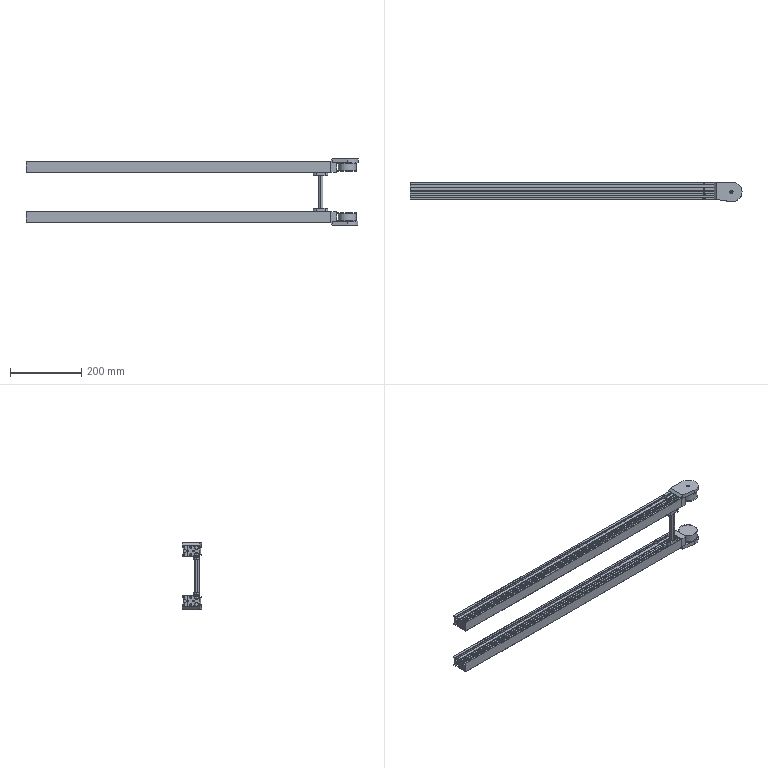Part | STEP file | Guide wheel mechanism revised.sldasm-Part-53 | 1 solid | 555 faces | box 932 x 54 x 186 mm | volume 1837685 mm3 | plane 438 | cylinder 105 | cone 12 | commonest cylinder face diameters 12.2 x16 54 x11 1 x8 5 x8 6 x8 6.4 x8